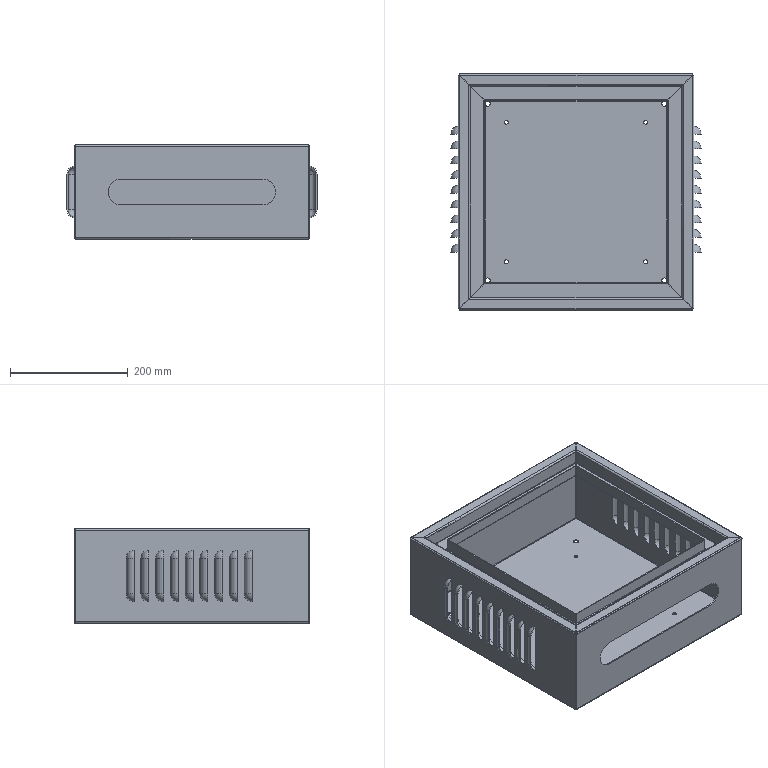Part | STEP file | panel body | 1 solid | 331 faces | box 424 x 400 x 160 mm | volume 948430 mm3 | plane 124 | cylinder 95 | sphere 72 | spline 40 | commonest cylinder face diameters 2 x20 5.6 x20 24 x18 27.6 x18 6.6 x8 9 x8